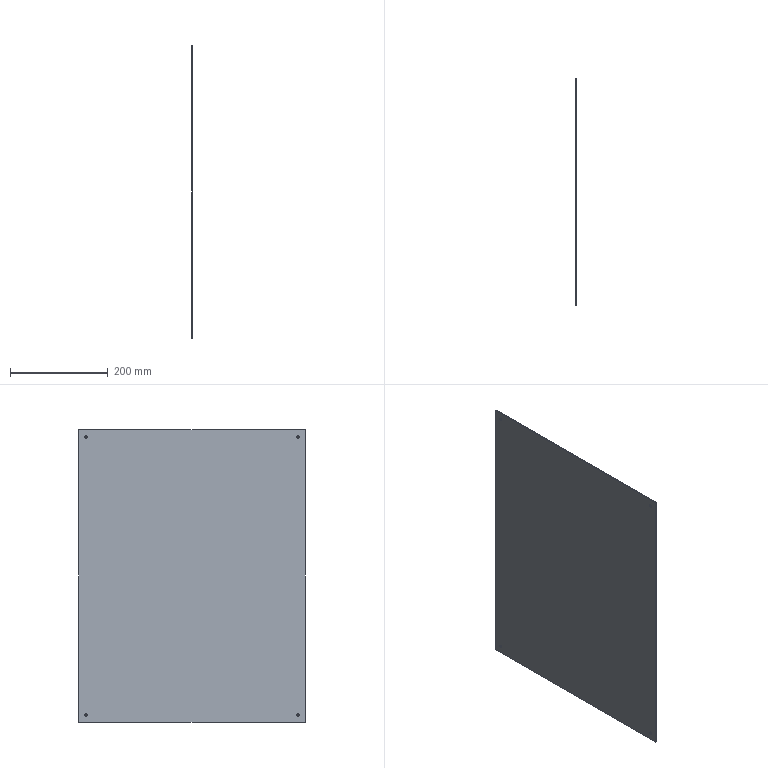Part | STEP file | PN_0056 (cover plate) | 1 solid | 14 faces | box 2 x 463 x 598 mm | volume 553591 mm3 | cylinder 8 | plane 6 | commonest cylinder face diameters 5 x8
STEP:
#1=CARTESIAN_POINT('',(0.,0.,0.));
#2=DIRECTION('',(0.,0.,1.));
#3=DIRECTION('',(1.,0.,0.));
#4=AXIS2_PLACEMENT_3D('',#1,#2,#3);
#5=CARTESIAN_POINT('',(-2.,216.5,281.5));
#6=VERTEX_POINT('',#5);
#7=CARTESIAN_POINT('',(0.,216.5,281.5));
#8=VERTEX_POINT('',#7);
#9=CARTESIAN_POINT('',(0.,216.5,281.5));
#10=DIRECTION('',(1.,0.,0.));
#11=VECTOR('',#10,1.);
#12=LINE('',#9,#11);
#13=CARTESIAN_POINT('',(0.,216.5,284.));
#14=DIRECTION('',(1.,0.,0.));
#15=DIRECTION('',(0.,0.,-1.));
#16=AXIS2_PLACEMENT_3D('',#13,#14,#15);
#17=CYLINDRICAL_SURFACE('',#16,2.5);
#18=CARTESIAN_POINT('',(6.283,0.));
#19=DIRECTION('',(0.,1.));
#20=VECTOR('',#19,1.);
#21=LINE('',#18,#20);
#22=(GEOMETRIC_REPRESENTATION_CONTEXT(2)PARAMETRIC_REPRESENTATION_CONTEXT()REPRESENTATION_CONTEXT('',''));
#23=DEFINITIONAL_REPRESENTATION('',(#21),#22);
#24=PCURVE('',#17,#23);
#25=CARTESIAN_POINT('',(0.,216.5,284.));
#26=DIRECTION('',(1.,0.,0.));
#27=DIRECTION('',(0.,0.,-1.));
#28=AXIS2_PLACEMENT_3D('',#25,#26,#27);
#29=CYLINDRICAL_SURFACE('',#28,2.5);
#30=CARTESIAN_POINT('',(0.,0.));
#31=DIRECTION('',(0.,1.));
#32=VECTOR('',#31,1.);
#33=LINE('',#30,#32);
#34=(GEOMETRIC_REPRESENTATION_CONTEXT(2)PARAMETRIC_REPRESENTATION_CONTEXT()REPRESENTATION_CONTEXT('',''));
#35=DEFINITIONAL_REPRESENTATION('',(#33),#34);
#36=PCURVE('',#29,#35);
#37=SURFACE_CURVE('',#12,(#24,#36),.PCURVE_S1.);
#38=EDGE_CURVE('',#6,#8,#37,.T.);
#39=ORIENTED_EDGE('',*,*,#38,.T.);
#40=CARTESIAN_POINT('',(0.,216.5,286.5));
#41=VERTEX_POINT('',#40);
#42=CARTESIAN_POINT('',(0.,216.5,284.));
#43=DIRECTION('',(1.,0.,0.));
#44=DIRECTION('',(0.,0.,-1.));
#45=AXIS2_PLACEMENT_3D('',#42,#43,#44);
#46=CIRCLE('',#45,2.5);
#47=CARTESIAN_POINT('',(0.,0.));
#48=DIRECTION('',(1.,0.));
#49=VECTOR('',#48,1.);
#50=LINE('',#47,#49);
#51=(GEOMETRIC_REPRESENTATION_CONTEXT(2)PARAMETRIC_REPRESENTATION_CONTEXT()REPRESENTATION_CONTEXT('',''));
#52=DEFINITIONAL_REPRESENTATION('',(#50),#51);
#53=PCURVE('',#17,#52);
#54=CARTESIAN_POINT('',(0.,0.,0.));
#55=DIRECTION('',(1.,0.,0.));
#56=DIRECTION('',(0.,0.,-1.));
#57=AXIS2_PLACEMENT_3D('',#54,#55,#56);
#58=PLANE('',#57);
#59=CARTESIAN_POINT('',(-284.,216.5));
#60=DIRECTION('',(1.,0.));
#61=AXIS2_PLACEMENT_2D('',#59,#60);
#62=CIRCLE('',#61,2.5);
#63=(GEOMETRIC_REPRESENTATION_CONTEXT(2)PARAMETRIC_REPRESENTATION_CONTEXT()REPRESENTATION_CONTEXT('',''));
#64=DEFINITIONAL_REPRESENTATION('',(#62),#63);
#65=PCURVE('',#58,#64);
#66=SURFACE_CURVE('',#46,(#53,#65),.PCURVE_S1.);
#67=EDGE_CURVE('',#41,#8,#66,.T.);
#68=ORIENTED_EDGE('',*,*,#67,.F.);
#69=CARTESIAN_POINT('',(-2.,216.5,286.5));
#70=VERTEX_POINT('',#69);
#71=CARTESIAN_POINT('',(0.,216.5,286.5));
#72=DIRECTION('',(1.,0.,0.));
#73=VECTOR('',#72,1.);
#74=LINE('',#71,#73);
#75=CARTESIAN_POINT('',(3.142,0.));
#76=DIRECTION('',(0.,1.));
#77=VECTOR('',#76,1.);
#78=LINE('',#75,#77);
#79=(GEOMETRIC_REPRESENTATION_CONTEXT(2)PARAMETRIC_REPRESENTATION_CONTEXT()REPRESENTATION_CONTEXT('',''));
#80=DEFINITIONAL_REPRESENTATION('',(#78),#79);
#81=PCURVE('',#17,#80);
#82=CARTESIAN_POINT('',(3.142,0.));
#83=DIRECTION('',(0.,1.));
#84=VECTOR('',#83,1.);
#85=LINE('',#82,#84);
#86=(GEOMETRIC_REPRESENTATION_CONTEXT(2)PARAMETRIC_REPRESENTATION_CONTEXT()REPRESENTATION_CONTEXT('',''));
#87=DEFINITIONAL_REPRESENTATION('',(#85),#86);
#88=PCURVE('',#29,#87);
#89=SURFACE_CURVE('',#74,(#81,#88),.PCURVE_S1.);
#90=EDGE_CURVE('',#70,#41,#89,.T.);
#91=ORIENTED_EDGE('',*,*,#90,.F.);
#92=CARTESIAN_POINT('',(-2.,216.5,284.));
#93=DIRECTION('',(1.,0.,0.));
#94=DIRECTION('',(0.,0.,-1.));
#95=AXIS2_PLACEMENT_3D('',#92,#93,#94);
#96=CIRCLE('',#95,2.5);
#97=CARTESIAN_POINT('',(0.,-2.));
#98=DIRECTION('',(1.,0.));
#99=VECTOR('',#98,1.);
#100=LINE('',#97,#99);
#101=(GEOMETRIC_REPRESENTATION_CONTEXT(2)PARAMETRIC_REPRESENTATION_CONTEXT()REPRESENTATION_CONTEXT('',''));
#102=DEFINITIONAL_REPRESENTATION('',(#100),#101);
#103=PCURVE('',#17,#102);
#104=CARTESIAN_POINT('',(-2.,0.,0.));
#105=DIRECTION('',(1.,0.,0.));
#106=DIRECTION('',(0.,0.,-1.));
#107=AXIS2_PLACEMENT_3D('',#104,#105,#106);
#108=PLANE('',#107);
#109=CARTESIAN_POINT('',(-284.,216.5));
#110=DIRECTION('',(1.,0.));
#111=AXIS2_PLACEMENT_2D('',#109,#110);
#112=CIRCLE('',#111,2.5);
#113=(GEOMETRIC_REPRESENTATION_CONTEXT(2)PARAMETRIC_REPRESENTATION_CONTEXT()REPRESENTATION_CONTEXT('',''));
#114=DEFINITIONAL_REPRESENTATION('',(#112),#113);
#115=PCURVE('',#108,#114);
#116=SURFACE_CURVE('',#96,(#103,#115),.PCURVE_S1.);
#117=EDGE_CURVE('',#70,#6,#116,.T.);
#118=ORIENTED_EDGE('',*,*,#117,.T.);
#119=EDGE_LOOP('',(#39,#68,#91,#118));
#120=FACE_BOUND('',#119,.F.);
#121=ADVANCED_FACE('',(#120),#17,.F.);
#122=CARTESIAN_POINT('',(-2.,-216.5,281.5));
#123=VERTEX_POINT('',#122);
#124=CARTESIAN_POINT('',(0.,-216.5,281.5));
#125=VERTEX_POINT('',#124);
#126=CARTESIAN_POINT('',(0.,-216.5,281.5));
#127=DIRECTION('',(1.,0.,0.));
#128=VECTOR('',#127,1.);
#129=LINE('',#126,#128);
#130=CARTESIAN_POINT('',(0.,-216.5,284.));
#131=DIRECTION('',(1.,0.,0.));
#132=DIRECTION('',(0.,0.,-1.));
#133=AXIS2_PLACEMENT_3D('',#130,#131,#132);
#134=CYLINDRICAL_SURFACE('',#133,2.5);
#135=CARTESIAN_POINT('',(6.283,0.));
#136=DIRECTION('',(0.,1.));
#137=VECTOR('',#136,1.);
#138=LINE('',#135,#137);
#139=(GEOMETRIC_REPRESENTATION_CONTEXT(2)PARAMETRIC_REPRESENTATION_CONTEXT()REPRESENTATION_CONTEXT('',''));
#140=DEFINITIONAL_REPRESENTATION('',(#138),#139);
#141=PCURVE('',#134,#140);
#142=CARTESIAN_POINT('',(0.,-216.5,284.));
#143=DIRECTION('',(1.,0.,0.));
#144=DIRECTION('',(0.,0.,-1.));
#145=AXIS2_PLACEMENT_3D('',#142,#143,#144);
#146=CYLINDRICAL_SURFACE('',#145,2.5);
#147=CARTESIAN_POINT('',(0.,0.));
#148=DIRECTION('',(0.,1.));
#149=VECTOR('',#148,1.);
#150=LINE('',#147,#149);
#151=(GEOMETRIC_REPRESENTATION_CONTEXT(2)PARAMETRIC_REPRESENTATION_CONTEXT()REPRESENTATION_CONTEXT('',''));
#152=DEFINITIONAL_REPRESENTATION('',(#150),#151);
#153=PCURVE('',#146,#152);
#154=SURFACE_CURVE('',#129,(#141,#153),.PCURVE_S1.);
#155=EDGE_CURVE('',#123,#125,#154,.T.);
#156=ORIENTED_EDGE('',*,*,#155,.T.);
#157=CARTESIAN_POINT('',(0.,-216.5,286.5));
#158=VERTEX_POINT('',#157);
#159=CARTESIAN_POINT('',(0.,-216.5,284.));
#160=DIRECTION('',(1.,0.,0.));
#161=DIRECTION('',(0.,0.,-1.));
#162=AXIS2_PLACEMENT_3D('',#159,#160,#161);
#163=CIRCLE('',#162,2.5);
#164=CARTESIAN_POINT('',(0.,0.));
#165=DIRECTION('',(1.,0.));
#166=VECTOR('',#165,1.);
#167=LINE('',#164,#166);
#168=(GEOMETRIC_REPRESENTATION_CONTEXT(2)PARAMETRIC_REPRESENTATION_CONTEXT()REPRESENTATION_CONTEXT('',''));
#169=DEFINITIONAL_REPRESENTATION('',(#167),#168);
#170=PCURVE('',#134,#169);
#171=CARTESIAN_POINT('',(-284.,-216.5));
#172=DIRECTION('',(1.,0.));
#173=AXIS2_PLACEMENT_2D('',#171,#172);
#174=CIRCLE('',#173,2.5);
#175=(GEOMETRIC_REPRESENTATION_CONTEXT(2)PARAMETRIC_REPRESENTATION_CONTEXT()REPRESENTATION_CONTEXT('',''));
#176=DEFINITIONAL_REPRESENTATION('',(#174),#175);
#177=PCURVE('',#58,#176);
#178=SURFACE_CURVE('',#163,(#170,#177),.PCURVE_S1.);
#179=EDGE_CURVE('',#158,#125,#178,.T.);
#180=ORIENTED_EDGE('',*,*,#179,.F.);
#181=CARTESIAN_POINT('',(-2.,-216.5,286.5));
#182=VERTEX_POINT('',#181);
#183=CARTESIAN_POINT('',(0.,-216.5,286.5));
#184=DIRECTION('',(1.,0.,0.));
#185=VECTOR('',#184,1.);
#186=LINE('',#183,#185);
#187=CARTESIAN_POINT('',(3.142,0.));
#188=DIRECTION('',(0.,1.));
#189=VECTOR('',#188,1.);
#190=LINE('',#187,#189);
#191=(GEOMETRIC_REPRESENTATION_CONTEXT(2)PARAMETRIC_REPRESENTATION_CONTEXT()REPRESENTATION_CONTEXT('',''));
#192=DEFINITIONAL_REPRESENTATION('',(#190),#191);
#193=PCURVE('',#134,#192);
#194=CARTESIAN_POINT('',(3.142,0.));
#195=DIRECTION('',(0.,1.));
#196=VECTOR('',#195,1.);
#197=LINE('',#194,#196);
#198=(GEOMETRIC_REPRESENTATION_CONTEXT(2)PARAMETRIC_REPRESENTATION_CONTEXT()REPRESENTATION_CONTEXT('',''));
#199=DEFINITIONAL_REPRESENTATION('',(#197),#198);
#200=PCURVE('',#146,#199);
#201=SURFACE_CURVE('',#186,(#193,#200),.PCURVE_S1.);
#202=EDGE_CURVE('',#182,#158,#201,.T.);
#203=ORIENTED_EDGE('',*,*,#202,.F.);
#204=CARTESIAN_POINT('',(-2.,-216.5,284.));
#205=DIRECTION('',(1.,0.,0.));
#206=DIRECTION('',(0.,0.,-1.));
#207=AXIS2_PLACEMENT_3D('',#204,#205,#206);
#208=CIRCLE('',#207,2.5);
#209=CARTESIAN_POINT('',(0.,-2.));
#210=DIRECTION('',(1.,0.));
#211=VECTOR('',#210,1.);
#212=LINE('',#209,#211);
#213=(GEOMETRIC_REPRESENTATION_CONTEXT(2)PARAMETRIC_REPRESENTATION_CONTEXT()REPRESENTATION_CONTEXT('',''));
#214=DEFINITIONAL_REPRESENTATION('',(#212),#213);
#215=PCURVE('',#134,#214);
#216=CARTESIAN_POINT('',(-284.,-216.5));
#217=DIRECTION('',(1.,0.));
#218=AXIS2_PLACEMENT_2D('',#216,#217);
#219=CIRCLE('',#218,2.5);
#220=(GEOMETRIC_REPRESENTATION_CONTEXT(2)PARAMETRIC_REPRESENTATION_CONTEXT()REPRESENTATION_CONTEXT('',''));
#221=DEFINITIONAL_REPRESENTATION('',(#219),#220);
#222=PCURVE('',#108,#221);
#223=SURFACE_CURVE('',#208,(#215,#222),.PCURVE_S1.);
#224=EDGE_CURVE('',#182,#123,#223,.T.);
#225=ORIENTED_EDGE('',*,*,#224,.T.);
#226=EDGE_LOOP('',(#156,#180,#203,#225));
#227=FACE_BOUND('',#226,.F.);
#228=ADVANCED_FACE('',(#227),#134,.F.);
#229=CARTESIAN_POINT('',(-2.,-216.5,-286.5));
#230=VERTEX_POINT('',#229);
#231=CARTESIAN_POINT('',(0.,-216.5,-286.5));
#232=VERTEX_POINT('',#231);
#233=CARTESIAN_POINT('',(0.,-216.5,-286.5));
#234=DIRECTION('',(1.,0.,0.));
#235=VECTOR('',#234,1.);
#236=LINE('',#233,#235);
#237=CARTESIAN_POINT('',(0.,-216.5,-284.));
#238=DIRECTION('',(1.,0.,0.));
#239=DIRECTION('',(0.,0.,-1.));
#240=AXIS2_PLACEMENT_3D('',#237,#238,#239);
#241=CYLINDRICAL_SURFACE('',#240,2.5);
#242=CARTESIAN_POINT('',(6.283,0.));
#243=DIRECTION('',(0.,1.));
#244=VECTOR('',#243,1.);
#245=LINE('',#242,#244);
#246=(GEOMETRIC_REPRESENTATION_CONTEXT(2)PARAMETRIC_REPRESENTATION_CONTEXT()REPRESENTATION_CONTEXT('',''));
#247=DEFINITIONAL_REPRESENTATION('',(#245),#246);
#248=PCURVE('',#241,#247);
#249=CARTESIAN_POINT('',(0.,-216.5,-284.));
#250=DIRECTION('',(1.,0.,0.));
#251=DIRECTION('',(0.,0.,-1.));
#252=AXIS2_PLACEMENT_3D('',#249,#250,#251);
#253=CYLINDRICAL_SURFACE('',#252,2.5);
#254=CARTESIAN_POINT('',(0.,0.));
#255=DIRECTION('',(0.,1.));
#256=VECTOR('',#255,1.);
#257=LINE('',#254,#256);
#258=(GEOMETRIC_REPRESENTATION_CONTEXT(2)PARAMETRIC_REPRESENTATION_CONTEXT()REPRESENTATION_CONTEXT('',''));
#259=DEFINITIONAL_REPRESENTATION('',(#257),#258);
#260=PCURVE('',#253,#259);
#261=SURFACE_CURVE('',#236,(#248,#260),.PCURVE_S1.);
#262=EDGE_CURVE('',#230,#232,#261,.T.);
#263=ORIENTED_EDGE('',*,*,#262,.T.);
#264=CARTESIAN_POINT('',(0.,-216.5,-281.5));
#265=VERTEX_POINT('',#264);
#266=CARTESIAN_POINT('',(0.,-216.5,-284.));
#267=DIRECTION('',(1.,0.,0.));
#268=DIRECTION('',(0.,0.,-1.));
#269=AXIS2_PLACEMENT_3D('',#266,#267,#268);
#270=CIRCLE('',#269,2.5);
#271=CARTESIAN_POINT('',(0.,0.));
#272=DIRECTION('',(1.,0.));
#273=VECTOR('',#272,1.);
#274=LINE('',#271,#273);
#275=(GEOMETRIC_REPRESENTATION_CONTEXT(2)PARAMETRIC_REPRESENTATION_CONTEXT()REPRESENTATION_CONTEXT('',''));
#276=DEFINITIONAL_REPRESENTATION('',(#274),#275);
#277=PCURVE('',#241,#276);
#278=CARTESIAN_POINT('',(284.,-216.5));
#279=DIRECTION('',(1.,0.));
#280=AXIS2_PLACEMENT_2D('',#278,#279);
#281=CIRCLE('',#280,2.5);
#282=(GEOMETRIC_REPRESENTATION_CONTEXT(2)PARAMETRIC_REPRESENTATION_CONTEXT()REPRESENTATION_CONTEXT('',''));
#283=DEFINITIONAL_REPRESENTATION('',(#281),#282);
#284=PCURVE('',#58,#283);
#285=SURFACE_CURVE('',#270,(#277,#284),.PCURVE_S1.);
#286=EDGE_CURVE('',#265,#232,#285,.T.);
#287=ORIENTED_EDGE('',*,*,#286,.F.);
#288=CARTESIAN_POINT('',(-2.,-216.5,-281.5));
#289=VERTEX_POINT('',#288);
#290=CARTESIAN_POINT('',(0.,-216.5,-281.5));
#291=DIRECTION('',(1.,0.,0.));
#292=VECTOR('',#291,1.);
#293=LINE('',#290,#292);
#294=CARTESIAN_POINT('',(3.142,0.));
#295=DIRECTION('',(0.,1.));
#296=VECTOR('',#295,1.);
#297=LINE('',#294,#296);
#298=(GEOMETRIC_REPRESENTATION_CONTEXT(2)PARAMETRIC_REPRESENTATION_CONTEXT()REPRESENTATION_CONTEXT('',''));
#299=DEFINITIONAL_REPRESENTATION('',(#297),#298);
#300=PCURVE('',#241,#299);
#301=CARTESIAN_POINT('',(3.142,0.));
#302=DIRECTION('',(0.,1.));
#303=VECTOR('',#302,1.);
#304=LINE('',#301,#303);
#305=(GEOMETRIC_REPRESENTATION_CONTEXT(2)PARAMETRIC_REPRESENTATION_CONTEXT()REPRESENTATION_CONTEXT('',''));
#306=DEFINITIONAL_REPRESENTATION('',(#304),#305);
#307=PCURVE('',#253,#306);
#308=SURFACE_CURVE('',#293,(#300,#307),.PCURVE_S1.);
#309=EDGE_CURVE('',#289,#265,#308,.T.);
#310=ORIENTED_EDGE('',*,*,#309,.F.);
#311=CARTESIAN_POINT('',(-2.,-216.5,-284.));
#312=DIRECTION('',(1.,0.,0.));
#313=DIRECTION('',(0.,0.,-1.));
#314=AXIS2_PLACEMENT_3D('',#311,#312,#313);
#315=CIRCLE('',#314,2.5);
#316=CARTESIAN_POINT('',(0.,-2.));
#317=DIRECTION('',(1.,0.));
#318=VECTOR('',#317,1.);
#319=LINE('',#316,#318);
#320=(GEOMETRIC_REPRESENTATION_CONTEXT(2)PARAMETRIC_REPRESENTATION_CONTEXT()REPRESENTATION_CONTEXT('',''));
#321=DEFINITIONAL_REPRESENTATION('',(#319),#320);
#322=PCURVE('',#241,#321);
#323=CARTESIAN_POINT('',(284.,-216.5));
#324=DIRECTION('',(1.,0.));
#325=AXIS2_PLACEMENT_2D('',#323,#324);
#326=CIRCLE('',#325,2.5);
#327=(GEOMETRIC_REPRESENTATION_CONTEXT(2)PARAMETRIC_REPRESENTATION_CONTEXT()REPRESENTATION_CONTEXT('',''));
#328=DEFINITIONAL_REPRESENTATION('',(#326),#327);
#329=PCURVE('',#108,#328);
#330=SURFACE_CURVE('',#315,(#322,#329),.PCURVE_S1.);
#331=EDGE_CURVE('',#289,#230,#330,.T.);
#332=ORIENTED_EDGE('',*,*,#331,.T.);
#333=EDGE_LOOP('',(#263,#287,#310,#332));
#334=FACE_BOUND('',#333,.F.);
#335=ADVANCED_FACE('',(#334),#241,.F.);
#336=CARTESIAN_POINT('',(-2.,216.5,-286.5));
#337=VERTEX_POINT('',#336);
#338=CARTESIAN_POINT('',(0.,216.5,-286.5));
#339=VERTEX_POINT('',#338);
#340=CARTESIAN_POINT('',(0.,216.5,-286.5));
#341=DIRECTION('',(1.,0.,0.));
#342=VECTOR('',#341,1.);
#343=LINE('',#340,#342);
#344=CARTESIAN_POINT('',(0.,216.5,-284.));
#345=DIRECTION('',(1.,0.,0.));
#346=DIRECTION('',(0.,0.,-1.));
#347=AXIS2_PLACEMENT_3D('',#344,#345,#346);
#348=CYLINDRICAL_SURFACE('',#347,2.5);
#349=CARTESIAN_POINT('',(6.283,0.));
#350=DIRECTION('',(0.,1.));
#351=VECTOR('',#350,1.);
#352=LINE('',#349,#351);
#353=(GEOMETRIC_REPRESENTATION_CONTEXT(2)PARAMETRIC_REPRESENTATION_CONTEXT()REPRESENTATION_CONTEXT('',''));
#354=DEFINITIONAL_REPRESENTATION('',(#352),#353);
#355=PCURVE('',#348,#354);
#356=CARTESIAN_POINT('',(0.,216.5,-284.));
#357=DIRECTION('',(1.,0.,0.));
#358=DIRECTION('',(0.,0.,-1.));
#359=AXIS2_PLACEMENT_3D('',#356,#357,#358);
#360=CYLINDRICAL_SURFACE('',#359,2.5);
#361=CARTESIAN_POINT('',(0.,0.));
#362=DIRECTION('',(0.,1.));
#363=VECTOR('',#362,1.);
#364=LINE('',#361,#363);
#365=(GEOMETRIC_REPRESENTATION_CONTEXT(2)PARAMETRIC_REPRESENTATION_CONTEXT()REPRESENTATION_CONTEXT('',''));
#366=DEFINITIONAL_REPRESENTATION('',(#364),#365);
#367=PCURVE('',#360,#366);
#368=SURFACE_CURVE('',#343,(#355,#367),.PCURVE_S1.);
#369=EDGE_CURVE('',#337,#339,#368,.T.);
#370=ORIENTED_EDGE('',*,*,#369,.T.);
#371=CARTESIAN_POINT('',(0.,216.5,-281.5));
#372=VERTEX_POINT('',#371);
#373=CARTESIAN_POINT('',(0.,216.5,-284.));
#374=DIRECTION('',(1.,0.,0.));
#375=DIRECTION('',(0.,0.,-1.));
#376=AXIS2_PLACEMENT_3D('',#373,#374,#375);
#377=CIRCLE('',#376,2.5);
#378=CARTESIAN_POINT('',(0.,0.));
#379=DIRECTION('',(1.,0.));
#380=VECTOR('',#379,1.);
#381=LINE('',#378,#380);
#382=(GEOMETRIC_REPRESENTATION_CONTEXT(2)PARAMETRIC_REPRESENTATION_CONTEXT()REPRESENTATION_CONTEXT('',''));
#383=DEFINITIONAL_REPRESENTATION('',(#381),#382);
#384=PCURVE('',#348,#383);
#385=CARTESIAN_POINT('',(284.,216.5));
#386=DIRECTION('',(1.,0.));
#387=AXIS2_PLACEMENT_2D('',#385,#386);
#388=CIRCLE('',#387,2.5);
#389=(GEOMETRIC_REPRESENTATION_CONTEXT(2)PARAMETRIC_REPRESENTATION_CONTEXT()REPRESENTATION_CONTEXT('',''));
#390=DEFINITIONAL_REPRESENTATION('',(#388),#389);
#391=PCURVE('',#58,#390);
#392=SURFACE_CURVE('',#377,(#384,#391),.PCURVE_S1.);
#393=EDGE_CURVE('',#372,#339,#392,.T.);
#394=ORIENTED_EDGE('',*,*,#393,.F.);
#395=CARTESIAN_POINT('',(-2.,216.5,-281.5));
#396=VERTEX_POINT('',#395);
#397=CARTESIAN_POINT('',(0.,216.5,-281.5));
#398=DIRECTION('',(1.,0.,0.));
#399=VECTOR('',#398,1.);
#400=LINE('',#397,#399);
#401=CARTESIAN_POINT('',(3.142,0.));
#402=DIRECTION('',(0.,1.));
#403=VECTOR('',#402,1.);
#404=LINE('',#401,#403);
#405=(GEOMETRIC_REPRESENTATION_CONTEXT(2)PARAMETRIC_REPRESENTATION_CONTEXT()REPRESENTATION_CONTEXT('',''));
#406=DEFINITIONAL_REPRESENTATION('',(#404),#405);
#407=PCURVE('',#348,#406);
#408=CARTESIAN_POINT('',(3.142,0.));
#409=DIRECTION('',(0.,1.));
#410=VECTOR('',#409,1.);
#411=LINE('',#408,#410);
#412=(GEOMETRIC_REPRESENTATION_CONTEXT(2)PARAMETRIC_REPRESENTATION_CONTEXT()REPRESENTATION_CONTEXT('',''));
#413=DEFINITIONAL_REPRESENTATION('',(#411),#412);
#414=PCURVE('',#360,#413);
#415=SURFACE_CURVE('',#400,(#407,#414),.PCURVE_S1.);
#416=EDGE_CURVE('',#396,#372,#415,.T.);
#417=ORIENTED_EDGE('',*,*,#416,.F.);
#418=CARTESIAN_POINT('',(-2.,216.5,-284.));
#419=DIRECTION('',(1.,0.,0.));
#420=DIRECTION('',(0.,0.,-1.));
#421=AXIS2_PLACEMENT_3D('',#418,#419,#420);
#422=CIRCLE('',#421,2.5);
#423=CARTESIAN_POINT('',(0.,-2.));
#424=DIRECTION('',(1.,0.));
#425=VECTOR('',#424,1.);
#426=LINE('',#423,#425);
#427=(GEOMETRIC_REPRESENTATION_CONTEXT(2)PARAMETRIC_REPRESENTATION_CONTEXT()REPRESENTATION_CONTEXT('',''));
#428=DEFINITIONAL_REPRESENTATION('',(#426),#427);
#429=PCURVE('',#348,#428);
#430=CARTESIAN_POINT('',(284.,216.5));
#431=DIRECTION('',(1.,0.));
#432=AXIS2_PLACEMENT_2D('',#430,#431);
#433=CIRCLE('',#432,2.5);
#434=(GEOMETRIC_REPRESENTATION_CONTEXT(2)PARAMETRIC_REPRESENTATION_CONTEXT()REPRESENTATION_CONTEXT('',''));
#435=DEFINITIONAL_REPRESENTATION('',(#433),#434);
#436=PCURVE('',#108,#435);
#437=SURFACE_CURVE('',#422,(#429,#436),.PCURVE_S1.);
#438=EDGE_CURVE('',#396,#337,#437,.T.);
#439=ORIENTED_EDGE('',*,*,#438,.T.);
#440=EDGE_LOOP('',(#370,#394,#417,#439));
#441=FACE_BOUND('',#440,.F.);
#442=ADVANCED_FACE('',(#441),#348,.F.);
#443=CARTESIAN_POINT('',(0.,231.5,299.));
#444=VERTEX_POINT('',#443);
#445=CARTESIAN_POINT('',(0.,-231.5,299.));
#446=VERTEX_POINT('',#445);
#447=CARTESIAN_POINT('',(0.,-231.5,299.));
#448=DIRECTION('',(0.,-1.,0.));
#449=VECTOR('',#448,1.);
#450=LINE('',#447,#449);
#451=CARTESIAN_POINT('',(-2.,-231.5,299.));
#452=DIRECTION('',(0.,0.,1.));
#453=DIRECTION('',(1.,0.,0.));
#454=AXIS2_PLACEMENT_3D('',#451,#452,#453);
#455=PLANE('',#454);
#456=CARTESIAN_POINT('',(2.,0.));
#457=DIRECTION('',(0.,-1.));
#458=VECTOR('',#457,1.);
#459=LINE('',#456,#458);
#460=(GEOMETRIC_REPRESENTATION_CONTEXT(2)PARAMETRIC_REPRESENTATION_CONTEXT()REPRESENTATION_CONTEXT('',''));
#461=DEFINITIONAL_REPRESENTATION('',(#459),#460);
#462=PCURVE('',#455,#461);
#463=CARTESIAN_POINT('',(-299.,-231.5));
#464=DIRECTION('',(0.,-1.));
#465=VECTOR('',#464,1.);
#466=LINE('',#463,#465);
#467=(GEOMETRIC_REPRESENTATION_CONTEXT(2)PARAMETRIC_REPRESENTATION_CONTEXT()REPRESENTATION_CONTEXT('',''));
#468=DEFINITIONAL_REPRESENTATION('',(#466),#467);
#469=PCURVE('',#58,#468);
#470=SURFACE_CURVE('',#450,(#462,#469),.PCURVE_S1.);
#471=EDGE_CURVE('',#444,#446,#470,.T.);
#472=ORIENTED_EDGE('',*,*,#471,.F.);
#473=CARTESIAN_POINT('',(-2.,231.5,299.));
#474=VERTEX_POINT('',#473);
#475=CARTESIAN_POINT('',(-2.,231.5,299.));
#476=DIRECTION('',(1.,0.,0.));
#477=VECTOR('',#476,1.);
#478=LINE('',#475,#477);
#479=CARTESIAN_POINT('',(0.,463.));
#480=DIRECTION('',(1.,0.));
#481=VECTOR('',#480,1.);
#482=LINE('',#479,#481);
#483=(GEOMETRIC_REPRESENTATION_CONTEXT(2)PARAMETRIC_REPRESENTATION_CONTEXT()REPRESENTATION_CONTEXT('',''));
#484=DEFINITIONAL_REPRESENTATION('',(#482),#483);
#485=PCURVE('',#455,#484);
#486=CARTESIAN_POINT('',(-2.,231.5,-299.));
#487=DIRECTION('',(0.,1.,0.));
#488=DIRECTION('',(0.,0.,1.));
#489=AXIS2_PLACEMENT_3D('',#486,#487,#488);
#490=PLANE('',#489);
#491=CARTESIAN_POINT('',(598.,0.));
#492=DIRECTION('',(0.,1.));
#493=VECTOR('',#492,1.);
#494=LINE('',#491,#493);
#495=(GEOMETRIC_REPRESENTATION_CONTEXT(2)PARAMETRIC_REPRESENTATION_CONTEXT()REPRESENTATION_CONTEXT('',''));
#496=DEFINITIONAL_REPRESENTATION('',(#494),#495);
#497=PCURVE('',#490,#496);
#498=SURFACE_CURVE('',#478,(#485,#497),.PCURVE_S1.);
#499=EDGE_CURVE('',#474,#444,#498,.T.);
#500=ORIENTED_EDGE('',*,*,#499,.F.);
#501=CARTESIAN_POINT('',(-2.,-231.5,299.));
#502=VERTEX_POINT('',#501);
#503=CARTESIAN_POINT('',(-2.,-231.5,299.));
#504=DIRECTION('',(0.,-1.,0.));
#505=VECTOR('',#504,1.);
#506=LINE('',#503,#505);
#507=CARTESIAN_POINT('',(0.,0.));
#508=DIRECTION('',(0.,-1.));
#509=VECTOR('',#508,1.);
#510=LINE('',#507,#509);
#511=(GEOMETRIC_REPRESENTATION_CONTEXT(2)PARAMETRIC_REPRESENTATION_CONTEXT()REPRESENTATION_CONTEXT('',''));
#512=DEFINITIONAL_REPRESENTATION('',(#510),#511);
#513=PCURVE('',#455,#512);
#514=CARTESIAN_POINT('',(-299.,-231.5));
#515=DIRECTION('',(0.,-1.));
#516=VECTOR('',#515,1.);
#517=LINE('',#514,#516);
#518=(GEOMETRIC_REPRESENTATION_CONTEXT(2)PARAMETRIC_REPRESENTATION_CONTEXT()REPRESENTATION_CONTEXT('',''));
#519=DEFINITIONAL_REPRESENTATION('',(#517),#518);
#520=PCURVE('',#108,#519);
#521=SURFACE_CURVE('',#506,(#513,#520),.PCURVE_S1.);
#522=EDGE_CURVE('',#474,#502,#521,.T.);
#523=ORIENTED_EDGE('',*,*,#522,.T.);
#524=CARTESIAN_POINT('',(-2.,-231.5,299.));
#525=DIRECTION('',(1.,0.,0.));
#526=VECTOR('',#525,1.);
#527=LINE('',#524,#526);
#528=CARTESIAN_POINT('',(0.,0.));
#529=DIRECTION('',(1.,0.));
#530=VECTOR('',#529,1.);
#531=LINE('',#528,#530);
#532=(GEOMETRIC_REPRESENTATION_CONTEXT(2)PARAMETRIC_REPRESENTATION_CONTEXT()REPRESENTATION_CONTEXT('',''));
#533=DEFINITIONAL_REPRESENTATION('',(#531),#532);
#534=PCURVE('',#455,#533);
#535=CARTESIAN_POINT('',(-2.,-231.5,-299.));
#536=DIRECTION('',(0.,-1.,0.));
#537=DIRECTION('',(0.,0.,-1.));
#538=AXIS2_PLACEMENT_3D('',#535,#536,#537);
#539=PLANE('',#538);
#540=CARTESIAN_POINT('',(-598.,0.));
#541=DIRECTION('',(0.,1.));
#542=VECTOR('',#541,1.);
#543=LINE('',#540,#542);
#544=(GEOMETRIC_REPRESENTATION_CONTEXT(2)PARAMETRIC_REPRESENTATION_CONTEXT()REPRESENTATION_CONTEXT('',''));
#545=DEFINITIONAL_REPRESENTATION('',(#543),#544);
#546=PCURVE('',#539,#545);
#547=SURFACE_CURVE('',#527,(#534,#546),.PCURVE_S1.);
#548=EDGE_CURVE('',#502,#446,#547,.T.);
#549=ORIENTED_EDGE('',*,*,#548,.T.);
#550=EDGE_LOOP('',(#472,#500,#523,#549));
#551=FACE_BOUND('',#550,.T.);
#552=ADVANCED_FACE('',(#551),#455,.T.);
#553=CARTESIAN_POINT('',(0.,231.5,-299.));
#554=VERTEX_POINT('',#553);
#555=CARTESIAN_POINT('',(0.,231.5,-299.));
#556=DIRECTION('',(0.,0.,1.));
#557=VECTOR('',#556,1.);
#558=LINE('',#555,#557);
#559=CARTESIAN_POINT('',(0.,2.));
#560=DIRECTION('',(1.,0.));
#561=VECTOR('',#560,1.);
#562=LINE('',#559,#561);
#563=(GEOMETRIC_REPRESENTATION_CONTEXT(2)PARAMETRIC_REPRESENTATION_CONTEXT()REPRESENTATION_CONTEXT('',''));
#564=DEFINITIONAL_REPRESENTATION('',(#562),#563);
#565=PCURVE('',#490,#564);
#566=CARTESIAN_POINT('',(299.,231.5));
#567=DIRECTION('',(-1.,0.));
#568=VECTOR('',#567,1.);
#569=LINE('',#566,#568);
#570=(GEOMETRIC_REPRESENTATION_CONTEXT(2)PARAMETRIC_REPRESENTATION_CONTEXT()REPRESENTATION_CONTEXT('',''));
#571=DEFINITIONAL_REPRESENTATION('',(#569),#570);
#572=PCURVE('',#58,#571);
#573=SURFACE_CURVE('',#558,(#565,#572),.PCURVE_S1.);
#574=EDGE_CURVE('',#554,#444,#573,.T.);
#575=ORIENTED_EDGE('',*,*,#574,.F.);
#576=CARTESIAN_POINT('',(-2.,231.5,-299.));
#577=VERTEX_POINT('',#576);
#578=CARTESIAN_POINT('',(-2.,231.5,-299.));
#579=DIRECTION('',(1.,0.,0.));
#580=VECTOR('',#579,1.);
#581=LINE('',#578,#580);
#582=CARTESIAN_POINT('',(0.,0.));
#583=DIRECTION('',(0.,1.));
#584=VECTOR('',#583,1.);
#585=LINE('',#582,#584);
#586=(GEOMETRIC_REPRESENTATION_CONTEXT(2)PARAMETRIC_REPRESENTATION_CONTEXT()REPRESENTATION_CONTEXT('',''));
#587=DEFINITIONAL_REPRESENTATION('',(#585),#586);
#588=PCURVE('',#490,#587);
#589=CARTESIAN_POINT('',(-2.,-231.5,-299.));
#590=DIRECTION('',(0.,0.,-1.));
#591=DIRECTION('',(-1.,0.,0.));
#592=AXIS2_PLACEMENT_3D('',#589,#590,#591);
#593=PLANE('',#592);
#594=CARTESIAN_POINT('',(0.,463.));
#595=DIRECTION('',(-1.,0.));
#596=VECTOR('',#595,1.);
#597=LINE('',#594,#596);
#598=(GEOMETRIC_REPRESENTATION_CONTEXT(2)PARAMETRIC_REPRESENTATION_CONTEXT()REPRESENTATION_CONTEXT('',''));
#599=DEFINITIONAL_REPRESENTATION('',(#597),#598);
#600=PCURVE('',#593,#599);
#601=SURFACE_CURVE('',#581,(#588,#600),.PCURVE_S1.);
#602=EDGE_CURVE('',#577,#554,#601,.T.);
#603=ORIENTED_EDGE('',*,*,#602,.F.);
#604=CARTESIAN_POINT('',(-2.,231.5,-299.));
#605=DIRECTION('',(0.,0.,1.));
#606=VECTOR('',#605,1.);
#607=LINE('',#604,#606);
#608=CARTESIAN_POINT('',(0.,0.));
#609=DIRECTION('',(1.,0.));
#610=VECTOR('',#609,1.);
#611=LINE('',#608,#610);
#612=(GEOMETRIC_REPRESENTATION_CONTEXT(2)PARAMETRIC_REPRESENTATION_CONTEXT()REPRESENTATION_CONTEXT('',''));
#613=DEFINITIONAL_REPRESENTATION('',(#611),#612);
#614=PCURVE('',#490,#613);
#615=CARTESIAN_POINT('',(299.,231.5));
#616=DIRECTION('',(-1.,0.));
#617=VECTOR('',#616,1.);
#618=LINE('',#615,#617);
#619=(GEOMETRIC_REPRESENTATION_CONTEXT(2)PARAMETRIC_REPRESENTATION_CONTEXT()REPRESENTATION_CONTEXT('',''));
#620=DEFINITIONAL_REPRESENTATION('',(#618),#619);
#621=PCURVE('',#108,#620);
#622=SURFACE_CURVE('',#607,(#614,#621),.PCURVE_S1.);
#623=EDGE_CURVE('',#577,#474,#622,.T.);
#624=ORIENTED_EDGE('',*,*,#623,.T.);
#625=ORIENTED_EDGE('',*,*,#499,.T.);
#626=EDGE_LOOP('',(#575,#603,#624,#625));
#627=FACE_BOUND('',#626,.T.);
#628=ADVANCED_FACE('',(#627),#490,.T.);
#629=CARTESIAN_POINT('',(0.,-231.5,-299.));
#630=VERTEX_POINT('',#629);
#631=CARTESIAN_POINT('',(0.,-231.5,-299.));
#632=DIRECTION('',(0.,1.,0.));
#633=VECTOR('',#632,1.);
#634=LINE('',#631,#633);
#635=CARTESIAN_POINT('',(-2.,0.));
#636=DIRECTION('',(0.,1.));
#637=VECTOR('',#636,1.);
#638=LINE('',#635,#637);
#639=(GEOMETRIC_REPRESENTATION_CONTEXT(2)PARAMETRIC_REPRESENTATION_CONTEXT()REPRESENTATION_CONTEXT('',''));
#640=DEFINITIONAL_REPRESENTATION('',(#638),#639);
#641=PCURVE('',#593,#640);
#642=CARTESIAN_POINT('',(299.,-231.5));
#643=DIRECTION('',(0.,1.));
#644=VECTOR('',#643,1.);
#645=LINE('',#642,#644);
#646=(GEOMETRIC_REPRESENTATION_CONTEXT(2)PARAMETRIC_REPRESENTATION_CONTEXT()REPRESENTATION_CONTEXT('',''));
#647=DEFINITIONAL_REPRESENTATION('',(#645),#646);
#648=PCURVE('',#58,#647);
#649=SURFACE_CURVE('',#634,(#641,#648),.PCURVE_S1.);
#650=EDGE_CURVE('',#630,#554,#649,.T.);
#651=ORIENTED_EDGE('',*,*,#650,.F.);
#652=CARTESIAN_POINT('',(-2.,-231.5,-299.));
#653=VERTEX_POINT('',#652);
#654=CARTESIAN_POINT('',(-2.,-231.5,-299.));
#655=DIRECTION('',(1.,0.,0.));
#656=VECTOR('',#655,1.);
#657=LINE('',#654,#656);
#658=CARTESIAN_POINT('',(0.,0.));
#659=DIRECTION('',(-1.,0.));
#660=VECTOR('',#659,1.);
#661=LINE('',#658,#660);
#662=(GEOMETRIC_REPRESENTATION_CONTEXT(2)PARAMETRIC_REPRESENTATION_CONTEXT()REPRESENTATION_CONTEXT('',''));
#663=DEFINITIONAL_REPRESENTATION('',(#661),#662);
#664=PCURVE('',#593,#663);
#665=CARTESIAN_POINT('',(0.,0.));
#666=DIRECTION('',(0.,1.));
#667=VECTOR('',#666,1.);
#668=LINE('',#665,#667);
#669=(GEOMETRIC_REPRESENTATION_CONTEXT(2)PARAMETRIC_REPRESENTATION_CONTEXT()REPRESENTATION_CONTEXT('',''));
#670=DEFINITIONAL_REPRESENTATION('',(#668),#669);
#671=PCURVE('',#539,#670);
#672=SURFACE_CURVE('',#657,(#664,#671),.PCURVE_S1.);
#673=EDGE_CURVE('',#653,#630,#672,.T.);
#674=ORIENTED_EDGE('',*,*,#673,.F.);
#675=CARTESIAN_POINT('',(-2.,-231.5,-299.));
#676=DIRECTION('',(0.,1.,0.));
#677=VECTOR('',#676,1.);
#678=LINE('',#675,#677);
#679=CARTESIAN_POINT('',(0.,0.));
#680=DIRECTION('',(0.,1.));
#681=VECTOR('',#680,1.);
#682=LINE('',#679,#681);
#683=(GEOMETRIC_REPRESENTATION_CONTEXT(2)PARAMETRIC_REPRESENTATION_CONTEXT()REPRESENTATION_CONTEXT('',''));
#684=DEFINITIONAL_REPRESENTATION('',(#682),#683);
#685=PCURVE('',#593,#684);
#686=CARTESIAN_POINT('',(299.,-231.5));
#687=DIRECTION('',(0.,1.));
#688=VECTOR('',#687,1.);
#689=LINE('',#686,#688);
#690=(GEOMETRIC_REPRESENTATION_CONTEXT(2)PARAMETRIC_REPRESENTATION_CONTEXT()REPRESENTATION_CONTEXT('',''));
#691=DEFINITIONAL_REPRESENTATION('',(#689),#690);
#692=PCURVE('',#108,#691);
#693=SURFACE_CURVE('',#678,(#685,#692),.PCURVE_S1.);
#694=EDGE_CURVE('',#653,#577,#693,.T.);
#695=ORIENTED_EDGE('',*,*,#694,.T.);
#696=ORIENTED_EDGE('',*,*,#602,.T.);
#697=EDGE_LOOP('',(#651,#674,#695,#696));
#698=FACE_BOUND('',#697,.T.);
#699=ADVANCED_FACE('',(#698),#593,.T.);
#700=CARTESIAN_POINT('',(0.,-231.5,-299.));
#701=DIRECTION('',(0.,0.,-1.));
#702=VECTOR('',#701,1.);
#703=LINE('',#700,#702);
#704=CARTESIAN_POINT('',(0.,2.));
#705=DIRECTION('',(1.,0.));
#706=VECTOR('',#705,1.);
#707=LINE('',#704,#706);
#708=(GEOMETRIC_REPRESENTATION_CONTEXT(2)PARAMETRIC_REPRESENTATION_CONTEXT()REPRESENTATION_CONTEXT('',''));
#709=DEFINITIONAL_REPRESENTATION('',(#707),#708);
#710=PCURVE('',#539,#709);
#711=CARTESIAN_POINT('',(299.,-231.5));
#712=DIRECTION('',(1.,0.));
#713=VECTOR('',#712,1.);
#714=LINE('',#711,#713);
#715=(GEOMETRIC_REPRESENTATION_CONTEXT(2)PARAMETRIC_REPRESENTATION_CONTEXT()REPRESENTATION_CONTEXT('',''));
#716=DEFINITIONAL_REPRESENTATION('',(#714),#715);
#717=PCURVE('',#58,#716);
#718=SURFACE_CURVE('',#703,(#710,#717),.PCURVE_S1.);
#719=EDGE_CURVE('',#446,#630,#718,.T.);
#720=ORIENTED_EDGE('',*,*,#719,.F.);
#721=ORIENTED_EDGE('',*,*,#548,.F.);
#722=CARTESIAN_POINT('',(-2.,-231.5,-299.));
#723=DIRECTION('',(0.,0.,-1.));
#724=VECTOR('',#723,1.);
#725=LINE('',#722,#724);
#726=CARTESIAN_POINT('',(0.,0.));
#727=DIRECTION('',(1.,0.));
#728=VECTOR('',#727,1.);
#729=LINE('',#726,#728);
#730=(GEOMETRIC_REPRESENTATION_CONTEXT(2)PARAMETRIC_REPRESENTATION_CONTEXT()REPRESENTATION_CONTEXT('',''));
#731=DEFINITIONAL_REPRESENTATION('',(#729),#730);
#732=PCURVE('',#539,#731);
#733=CARTESIAN_POINT('',(299.,-231.5));
#734=DIRECTION('',(1.,0.));
#735=VECTOR('',#734,1.);
#736=LINE('',#733,#735);
#737=(GEOMETRIC_REPRESENTATION_CONTEXT(2)PARAMETRIC_REPRESENTATION_CONTEXT()REPRESENTATION_CONTEXT('',''));
#738=DEFINITIONAL_REPRESENTATION('',(#736),#737);
#739=PCURVE('',#108,#738);
#740=SURFACE_CURVE('',#725,(#732,#739),.PCURVE_S1.);
#741=EDGE_CURVE('',#502,#653,#740,.T.);
#742=ORIENTED_EDGE('',*,*,#741,.T.);
#743=ORIENTED_EDGE('',*,*,#673,.T.);
#744=EDGE_LOOP('',(#720,#721,#742,#743));
#745=FACE_BOUND('',#744,.T.);
#746=ADVANCED_FACE('',(#745),#539,.T.);
#747=CARTESIAN_POINT('',(-2.,216.5,284.));
#748=DIRECTION('',(1.,0.,0.));
#749=DIRECTION('',(0.,0.,-1.));
#750=AXIS2_PLACEMENT_3D('',#747,#748,#749);
#751=CIRCLE('',#750,2.5);
#752=CARTESIAN_POINT('',(-284.,216.5));
#753=DIRECTION('',(1.,0.));
#754=AXIS2_PLACEMENT_2D('',#752,#753);
#755=CIRCLE('',#754,2.5);
#756=(GEOMETRIC_REPRESENTATION_CONTEXT(2)PARAMETRIC_REPRESENTATION_CONTEXT()REPRESENTATION_CONTEXT('',''));
#757=DEFINITIONAL_REPRESENTATION('',(#755),#756);
#758=PCURVE('',#108,#757);
#759=CARTESIAN_POINT('',(0.,-2.));
#760=DIRECTION('',(1.,0.));
#761=VECTOR('',#760,1.);
#762=LINE('',#759,#761);
#763=(GEOMETRIC_REPRESENTATION_CONTEXT(2)PARAMETRIC_REPRESENTATION_CONTEXT()REPRESENTATION_CONTEXT('',''));
#764=DEFINITIONAL_REPRESENTATION('',(#762),#763);
#765=PCURVE('',#29,#764);
#766=SURFACE_CURVE('',#751,(#758,#765),.PCURVE_S1.);
#767=EDGE_CURVE('',#6,#70,#766,.T.);
#768=ORIENTED_EDGE('',*,*,#767,.T.);
#769=ORIENTED_EDGE('',*,*,#117,.T.);
#770=EDGE_LOOP('',(#768,#769));
#771=FACE_BOUND('',#770,.T.);
#772=CARTESIAN_POINT('',(-2.,-216.5,284.));
#773=DIRECTION('',(1.,0.,0.));
#774=DIRECTION('',(0.,0.,-1.));
#775=AXIS2_PLACEMENT_3D('',#772,#773,#774);
#776=CIRCLE('',#775,2.5);
#777=CARTESIAN_POINT('',(-284.,-216.5));
#778=DIRECTION('',(1.,0.));
#779=AXIS2_PLACEMENT_2D('',#777,#778);
#780=CIRCLE('',#779,2.5);
#781=(GEOMETRIC_REPRESENTATION_CONTEXT(2)PARAMETRIC_REPRESENTATION_CONTEXT()REPRESENTATION_CONTEXT('',''));
#782=DEFINITIONAL_REPRESENTATION('',(#780),#781);
#783=PCURVE('',#108,#782);
#784=CARTESIAN_POINT('',(0.,-2.));
#785=DIRECTION('',(1.,0.));
#786=VECTOR('',#785,1.);
#787=LINE('',#784,#786);
#788=(GEOMETRIC_REPRESENTATION_CONTEXT(2)PARAMETRIC_REPRESENTATION_CONTEXT()REPRESENTATION_CONTEXT('',''));
#789=DEFINITIONAL_REPRESENTATION('',(#787),#788);
#790=PCURVE('',#146,#789);
#791=SURFACE_CURVE('',#776,(#783,#790),.PCURVE_S1.);
#792=EDGE_CURVE('',#123,#182,#791,.T.);
#793=ORIENTED_EDGE('',*,*,#792,.T.);
#794=ORIENTED_EDGE('',*,*,#224,.T.);
#795=EDGE_LOOP('',(#793,#794));
#796=FACE_BOUND('',#795,.T.);
#797=CARTESIAN_POINT('',(-2.,-216.5,-284.));
#798=DIRECTION('',(1.,0.,0.));
#799=DIRECTION('',(0.,0.,-1.));
#800=AXIS2_PLACEMENT_3D('',#797,#798,#799);
#801=CIRCLE('',#800,2.5);
#802=CARTESIAN_POINT('',(284.,-216.5));
#803=DIRECTION('',(1.,0.));
#804=AXIS2_PLACEMENT_2D('',#802,#803);
#805=CIRCLE('',#804,2.5);
#806=(GEOMETRIC_REPRESENTATION_CONTEXT(2)PARAMETRIC_REPRESENTATION_CONTEXT()REPRESENTATION_CONTEXT('',''));
#807=DEFINITIONAL_REPRESENTATION('',(#805),#806);
#808=PCURVE('',#108,#807);
#809=CARTESIAN_POINT('',(0.,-2.));
#810=DIRECTION('',(1.,0.));
#811=VECTOR('',#810,1.);
#812=LINE('',#809,#811);
#813=(GEOMETRIC_REPRESENTATION_CONTEXT(2)PARAMETRIC_REPRESENTATION_CONTEXT()REPRESENTATION_CONTEXT('',''));
#814=DEFINITIONAL_REPRESENTATION('',(#812),#813);
#815=PCURVE('',#253,#814);
#816=SURFACE_CURVE('',#801,(#808,#815),.PCURVE_S1.);
#817=EDGE_CURVE('',#230,#289,#816,.T.);
#818=ORIENTED_EDGE('',*,*,#817,.T.);
#819=ORIENTED_EDGE('',*,*,#331,.T.);
#820=EDGE_LOOP('',(#818,#819));
#821=FACE_BOUND('',#820,.T.);
#822=CARTESIAN_POINT('',(-2.,216.5,-284.));
#823=DIRECTION('',(1.,0.,0.));
#824=DIRECTION('',(0.,0.,-1.));
#825=AXIS2_PLACEMENT_3D('',#822,#823,#824);
#826=CIRCLE('',#825,2.5);
#827=CARTESIAN_POINT('',(284.,216.5));
#828=DIRECTION('',(1.,0.));
#829=AXIS2_PLACEMENT_2D('',#827,#828);
#830=CIRCLE('',#829,2.5);
#831=(GEOMETRIC_REPRESENTATION_CONTEXT(2)PARAMETRIC_REPRESENTATION_CONTEXT()REPRESENTATION_CONTEXT('',''));
#832=DEFINITIONAL_REPRESENTATION('',(#830),#831);
#833=PCURVE('',#108,#832);
#834=CARTESIAN_POINT('',(0.,-2.));
#835=DIRECTION('',(1.,0.));
#836=VECTOR('',#835,1.);
#837=LINE('',#834,#836);
#838=(GEOMETRIC_REPRESENTATION_CONTEXT(2)PARAMETRIC_REPRESENTATION_CONTEXT()REPRESENTATION_CONTEXT('',''));
#839=DEFINITIONAL_REPRESENTATION('',(#837),#838);
#840=PCURVE('',#360,#839);
#841=SURFACE_CURVE('',#826,(#833,#840),.PCURVE_S1.);
#842=EDGE_CURVE('',#337,#396,#841,.T.);
#843=ORIENTED_EDGE('',*,*,#842,.T.);
#844=ORIENTED_EDGE('',*,*,#438,.T.);
#845=EDGE_LOOP('',(#843,#844));
#846=FACE_BOUND('',#845,.T.);
#847=ORIENTED_EDGE('',*,*,#522,.F.);
#848=ORIENTED_EDGE('',*,*,#623,.F.);
#849=ORIENTED_EDGE('',*,*,#694,.F.);
#850=ORIENTED_EDGE('',*,*,#741,.F.);
#851=EDGE_LOOP('',(#847,#848,#849,#850));
#852=FACE_BOUND('',#851,.T.);
#853=ADVANCED_FACE('',(#771,#796,#821,#846,#852),#108,.F.);
#854=CARTESIAN_POINT('',(0.,216.5,284.));
#855=DIRECTION('',(1.,0.,0.));
#856=DIRECTION('',(0.,0.,-1.));
#857=AXIS2_PLACEMENT_3D('',#854,#855,#856);
#858=CIRCLE('',#857,2.5);
#859=CARTESIAN_POINT('',(-284.,216.5));
#860=DIRECTION('',(1.,0.));
#861=AXIS2_PLACEMENT_2D('',#859,#860);
#862=CIRCLE('',#861,2.5);
#863=(GEOMETRIC_REPRESENTATION_CONTEXT(2)PARAMETRIC_REPRESENTATION_CONTEXT()REPRESENTATION_CONTEXT('',''));
#864=DEFINITIONAL_REPRESENTATION('',(#862),#863);
#865=PCURVE('',#58,#864);
#866=CARTESIAN_POINT('',(0.,0.));
#867=DIRECTION('',(1.,0.));
#868=VECTOR('',#867,1.);
#869=LINE('',#866,#868);
#870=(GEOMETRIC_REPRESENTATION_CONTEXT(2)PARAMETRIC_REPRESENTATION_CONTEXT()REPRESENTATION_CONTEXT('',''));
#871=DEFINITIONAL_REPRESENTATION('',(#869),#870);
#872=PCURVE('',#29,#871);
#873=SURFACE_CURVE('',#858,(#865,#872),.PCURVE_S1.);
#874=EDGE_CURVE('',#8,#41,#873,.T.);
#875=ORIENTED_EDGE('',*,*,#874,.F.);
#876=ORIENTED_EDGE('',*,*,#67,.F.);
#877=EDGE_LOOP('',(#875,#876));
#878=FACE_BOUND('',#877,.T.);
#879=CARTESIAN_POINT('',(0.,-216.5,284.));
#880=DIRECTION('',(1.,0.,0.));
#881=DIRECTION('',(0.,0.,-1.));
#882=AXIS2_PLACEMENT_3D('',#879,#880,#881);
#883=CIRCLE('',#882,2.5);
#884=CARTESIAN_POINT('',(-284.,-216.5));
#885=DIRECTION('',(1.,0.));
#886=AXIS2_PLACEMENT_2D('',#884,#885);
#887=CIRCLE('',#886,2.5);
#888=(GEOMETRIC_REPRESENTATION_CONTEXT(2)PARAMETRIC_REPRESENTATION_CONTEXT()REPRESENTATION_CONTEXT('',''));
#889=DEFINITIONAL_REPRESENTATION('',(#887),#888);
#890=PCURVE('',#58,#889);
#891=CARTESIAN_POINT('',(0.,0.));
#892=DIRECTION('',(1.,0.));
#893=VECTOR('',#892,1.);
#894=LINE('',#891,#893);
#895=(GEOMETRIC_REPRESENTATION_CONTEXT(2)PARAMETRIC_REPRESENTATION_CONTEXT()REPRESENTATION_CONTEXT('',''));
#896=DEFINITIONAL_REPRESENTATION('',(#894),#895);
#897=PCURVE('',#146,#896);
#898=SURFACE_CURVE('',#883,(#890,#897),.PCURVE_S1.);
#899=EDGE_CURVE('',#125,#158,#898,.T.);
#900=ORIENTED_EDGE('',*,*,#899,.F.);
#901=ORIENTED_EDGE('',*,*,#179,.F.);
#902=EDGE_LOOP('',(#900,#901));
#903=FACE_BOUND('',#902,.T.);
#904=CARTESIAN_POINT('',(0.,-216.5,-284.));
#905=DIRECTION('',(1.,0.,0.));
#906=DIRECTION('',(0.,0.,-1.));
#907=AXIS2_PLACEMENT_3D('',#904,#905,#906);
#908=CIRCLE('',#907,2.5);
#909=CARTESIAN_POINT('',(284.,-216.5));
#910=DIRECTION('',(1.,0.));
#911=AXIS2_PLACEMENT_2D('',#909,#910);
#912=CIRCLE('',#911,2.5);
#913=(GEOMETRIC_REPRESENTATION_CONTEXT(2)PARAMETRIC_REPRESENTATION_CONTEXT()REPRESENTATION_CONTEXT('',''));
#914=DEFINITIONAL_REPRESENTATION('',(#912),#913);
#915=PCURVE('',#58,#914);
#916=CARTESIAN_POINT('',(0.,0.));
#917=DIRECTION('',(1.,0.));
#918=VECTOR('',#917,1.);
#919=LINE('',#916,#918);
#920=(GEOMETRIC_REPRESENTATION_CONTEXT(2)PARAMETRIC_REPRESENTATION_CONTEXT()REPRESENTATION_CONTEXT('',''));
#921=DEFINITIONAL_REPRESENTATION('',(#919),#920);
#922=PCURVE('',#253,#921);
#923=SURFACE_CURVE('',#908,(#915,#922),.PCURVE_S1.);
#924=EDGE_CURVE('',#232,#265,#923,.T.);
#925=ORIENTED_EDGE('',*,*,#924,.F.);
#926=ORIENTED_EDGE('',*,*,#286,.F.);
#927=EDGE_LOOP('',(#925,#926));
#928=FACE_BOUND('',#927,.T.);
#929=CARTESIAN_POINT('',(0.,216.5,-284.));
#930=DIRECTION('',(1.,0.,0.));
#931=DIRECTION('',(0.,0.,-1.));
#932=AXIS2_PLACEMENT_3D('',#929,#930,#931);
#933=CIRCLE('',#932,2.5);
#934=CARTESIAN_POINT('',(284.,216.5));
#935=DIRECTION('',(1.,0.));
#936=AXIS2_PLACEMENT_2D('',#934,#935);
#937=CIRCLE('',#936,2.5);
#938=(GEOMETRIC_REPRESENTATION_CONTEXT(2)PARAMETRIC_REPRESENTATION_CONTEXT()REPRESENTATION_CONTEXT('',''));
#939=DEFINITIONAL_REPRESENTATION('',(#937),#938);
#940=PCURVE('',#58,#939);
#941=CARTESIAN_POINT('',(0.,0.));
#942=DIRECTION('',(1.,0.));
#943=VECTOR('',#942,1.);
#944=LINE('',#941,#943);
#945=(GEOMETRIC_REPRESENTATION_CONTEXT(2)PARAMETRIC_REPRESENTATION_CONTEXT()REPRESENTATION_CONTEXT('',''));
#946=DEFINITIONAL_REPRESENTATION('',(#944),#945);
#947=PCURVE('',#360,#946);
#948=SURFACE_CURVE('',#933,(#940,#947),.PCURVE_S1.);
#949=EDGE_CURVE('',#339,#372,#948,.T.);
#950=ORIENTED_EDGE('',*,*,#949,.F.);
#951=ORIENTED_EDGE('',*,*,#393,.F.);
#952=EDGE_LOOP('',(#950,#951));
#953=FACE_BOUND('',#952,.T.);
#954=ORIENTED_EDGE('',*,*,#471,.T.);
#955=ORIENTED_EDGE('',*,*,#719,.T.);
#956=ORIENTED_EDGE('',*,*,#650,.T.);
#957=ORIENTED_EDGE('',*,*,#574,.T.);
#958=EDGE_LOOP('',(#954,#955,#956,#957));
#959=FACE_BOUND('',#958,.T.);
#960=ADVANCED_FACE('',(#878,#903,#928,#953,#959),#58,.T.);
#961=ORIENTED_EDGE('',*,*,#949,.F.);
#962=ORIENTED_EDGE('',*,*,#369,.F.);
#963=ORIENTED_EDGE('',*,*,#842,.T.);
#964=ORIENTED_EDGE('',*,*,#416,.T.);
#965=EDGE_LOOP('',(#961,#962,#963,#964));
#966=FACE_BOUND('',#965,.F.);
#967=ADVANCED_FACE('',(#966),#360,.F.);
#968=ORIENTED_EDGE('',*,*,#924,.F.);
#969=ORIENTED_EDGE('',*,*,#262,.F.);
#970=ORIENTED_EDGE('',*,*,#817,.T.);
#971=ORIENTED_EDGE('',*,*,#309,.T.);
#972=EDGE_LOOP('',(#968,#969,#970,#971));
#973=FACE_BOUND('',#972,.F.);
#974=ADVANCED_FACE('',(#973),#253,.F.);
#975=ORIENTED_EDGE('',*,*,#899,.F.);
#976=ORIENTED_EDGE('',*,*,#155,.F.);
#977=ORIENTED_EDGE('',*,*,#792,.T.);
#978=ORIENTED_EDGE('',*,*,#202,.T.);
#979=EDGE_LOOP('',(#975,#976,#977,#978));
#980=FACE_BOUND('',#979,.F.);
#981=ADVANCED_FACE('',(#980),#146,.F.);
#982=ORIENTED_EDGE('',*,*,#874,.F.);
#983=ORIENTED_EDGE('',*,*,#38,.F.);
#984=ORIENTED_EDGE('',*,*,#767,.T.);
#985=ORIENTED_EDGE('',*,*,#90,.T.);
#986=EDGE_LOOP('',(#982,#983,#984,#985));
#987=FACE_BOUND('',#986,.F.);
#988=ADVANCED_FACE('',(#987),#29,.F.);
#989=CLOSED_SHELL('',(#121,#228,#335,#442,#552,#628,#699,#746,#853,#960,#967,#974,#981,#988));
#990=MANIFOLD_SOLID_BREP('',#989);
#991=(LENGTH_UNIT()NAMED_UNIT(*)SI_UNIT(.MILLI.,.METRE.));
#992=UNCERTAINTY_MEASURE_WITH_UNIT(LENGTH_MEASURE(0.0000001),#991,'','');
#993=(NAMED_UNIT(*)PLANE_ANGLE_UNIT()SI_UNIT($,.RADIAN.));
#994=(NAMED_UNIT(*)SI_UNIT($,.STERADIAN.)SOLID_ANGLE_UNIT());
#995=(GEOMETRIC_REPRESENTATION_CONTEXT(3)GLOBAL_UNCERTAINTY_ASSIGNED_CONTEXT((#992))GLOBAL_UNIT_ASSIGNED_CONTEXT((#991,#993,#994))REPRESENTATION_CONTEXT('',''));
#996=ADVANCED_BREP_SHAPE_REPRESENTATION('',(#4,#990),#995);